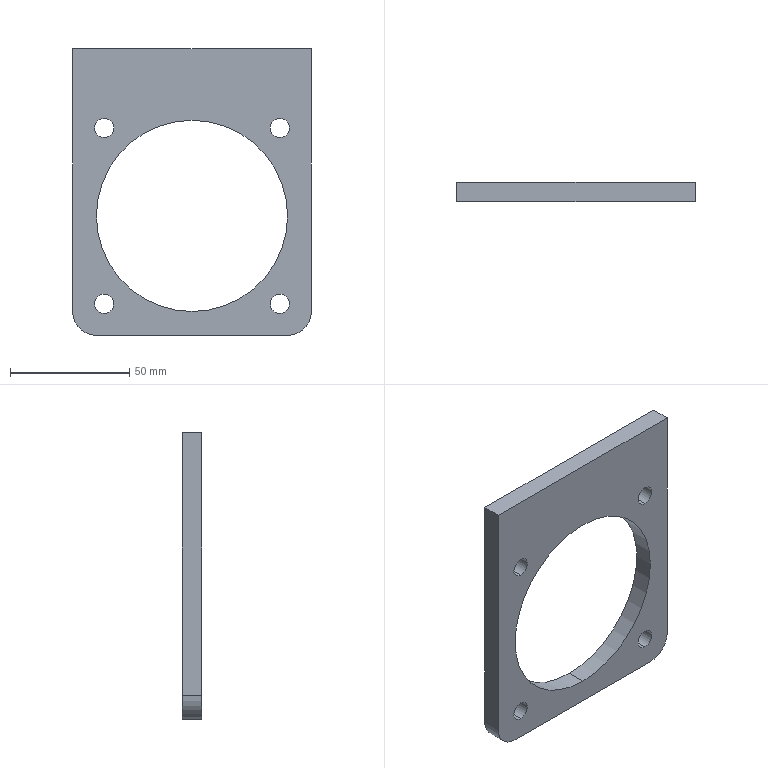Part | SolidWorks | features CirPattern 1, Extrusion 1, Fillet 1, HoleWzd 1, ICE 1 | 1 solid | 18 faces | box 100 x 8 x 120 mm | volume 53836 mm3 | cylinder 12 | plane 6 | commonest cylinder face diameters 8 x8 20 x2 80 x2
STEP:
#1=CARTESIAN_POINT('',(36.77,0.,-50.77));
#2=VERTEX_POINT('',#1);
#3=CARTESIAN_POINT('',(36.77,0.,-42.77));
#4=VERTEX_POINT('',#3);
#5=CARTESIAN_POINT('',(36.77,0.,-46.77));
#6=DIRECTION('',(0.,1.,0.));
#7=DIRECTION('',(0.,0.,1.));
#8=AXIS2_PLACEMENT_3D('',#5,#6,#7);
#9=CIRCLE('',#8,4.);
#10=EDGE_CURVE('',#2,#4,#9,.T.);
#11=ORIENTED_EDGE('',*,*,#10,.F.);
#12=CARTESIAN_POINT('',(36.77,8.,-50.77));
#13=VERTEX_POINT('',#12);
#14=CARTESIAN_POINT('',(36.77,8.,-50.77));
#15=DIRECTION('',(0.,1.,0.));
#16=VECTOR('',#15,1000.);
#17=LINE('',#14,#16);
#18=EDGE_CURVE('',#2,#13,#17,.T.);
#19=ORIENTED_EDGE('',*,*,#18,.T.);
#20=CARTESIAN_POINT('',(36.77,8.,-42.77));
#21=VERTEX_POINT('',#20);
#22=CARTESIAN_POINT('',(36.77,8.,-46.77));
#23=DIRECTION('',(0.,1.,0.));
#24=DIRECTION('',(0.,0.,1.));
#25=AXIS2_PLACEMENT_3D('',#22,#23,#24);
#26=CIRCLE('',#25,4.);
#27=EDGE_CURVE('',#13,#21,#26,.T.);
#28=ORIENTED_EDGE('',*,*,#27,.T.);
#29=CARTESIAN_POINT('',(36.77,8.,-42.77));
#30=DIRECTION('',(0.,1.,0.));
#31=VECTOR('',#30,1000.);
#32=LINE('',#29,#31);
#33=EDGE_CURVE('',#4,#21,#32,.T.);
#34=ORIENTED_EDGE('',*,*,#33,.F.);
#35=EDGE_LOOP('',(#11,#19,#28,#34));
#36=FACE_OUTER_BOUND('',#35,.T.);
#37=CARTESIAN_POINT('',(36.77,8.,-46.77));
#38=DIRECTION('',(0.,1.,0.));
#39=DIRECTION('',(0.,0.,1.));
#40=AXIS2_PLACEMENT_3D('',#37,#38,#39);
#41=CYLINDRICAL_SURFACE('',#40,4.);
#42=ADVANCED_FACE('',(#36),#41,.F.);
#43=CARTESIAN_POINT('',(36.77,0.,22.77));
#44=VERTEX_POINT('',#43);
#45=CARTESIAN_POINT('',(36.77,0.,30.77));
#46=VERTEX_POINT('',#45);
#47=CARTESIAN_POINT('',(36.77,0.,26.77));
#48=DIRECTION('',(0.,1.,0.));
#49=DIRECTION('',(0.,0.,1.));
#50=AXIS2_PLACEMENT_3D('',#47,#48,#49);
#51=CIRCLE('',#50,4.);
#52=EDGE_CURVE('',#44,#46,#51,.T.);
#53=ORIENTED_EDGE('',*,*,#52,.F.);
#54=CARTESIAN_POINT('',(36.77,8.,22.77));
#55=VERTEX_POINT('',#54);
#56=CARTESIAN_POINT('',(36.77,8.,22.77));
#57=DIRECTION('',(0.,1.,0.));
#58=VECTOR('',#57,1000.);
#59=LINE('',#56,#58);
#60=EDGE_CURVE('',#44,#55,#59,.T.);
#61=ORIENTED_EDGE('',*,*,#60,.T.);
#62=CARTESIAN_POINT('',(36.77,8.,30.77));
#63=VERTEX_POINT('',#62);
#64=CARTESIAN_POINT('',(36.77,8.,26.77));
#65=DIRECTION('',(0.,1.,0.));
#66=DIRECTION('',(0.,0.,1.));
#67=AXIS2_PLACEMENT_3D('',#64,#65,#66);
#68=CIRCLE('',#67,4.);
#69=EDGE_CURVE('',#55,#63,#68,.T.);
#70=ORIENTED_EDGE('',*,*,#69,.T.);
#71=CARTESIAN_POINT('',(36.77,8.,30.77));
#72=DIRECTION('',(0.,1.,0.));
#73=VECTOR('',#72,1000.);
#74=LINE('',#71,#73);
#75=EDGE_CURVE('',#46,#63,#74,.T.);
#76=ORIENTED_EDGE('',*,*,#75,.F.);
#77=EDGE_LOOP('',(#53,#61,#70,#76));
#78=FACE_OUTER_BOUND('',#77,.T.);
#79=CARTESIAN_POINT('',(36.77,8.,26.77));
#80=DIRECTION('',(0.,1.,0.));
#81=DIRECTION('',(0.,0.,1.));
#82=AXIS2_PLACEMENT_3D('',#79,#80,#81);
#83=CYLINDRICAL_SURFACE('',#82,4.);
#84=ADVANCED_FACE('',(#78),#83,.F.);
#85=CARTESIAN_POINT('',(-36.77,0.,22.77));
#86=VERTEX_POINT('',#85);
#87=CARTESIAN_POINT('',(-36.77,0.,30.77));
#88=VERTEX_POINT('',#87);
#89=CARTESIAN_POINT('',(-36.77,0.,26.77));
#90=DIRECTION('',(0.,1.,0.));
#91=DIRECTION('',(0.,0.,1.));
#92=AXIS2_PLACEMENT_3D('',#89,#90,#91);
#93=CIRCLE('',#92,4.);
#94=EDGE_CURVE('',#86,#88,#93,.T.);
#95=ORIENTED_EDGE('',*,*,#94,.F.);
#96=CARTESIAN_POINT('',(-36.77,8.,22.77));
#97=VERTEX_POINT('',#96);
#98=CARTESIAN_POINT('',(-36.77,8.,22.77));
#99=DIRECTION('',(0.,1.,0.));
#100=VECTOR('',#99,1000.);
#101=LINE('',#98,#100);
#102=EDGE_CURVE('',#86,#97,#101,.T.);
#103=ORIENTED_EDGE('',*,*,#102,.T.);
#104=CARTESIAN_POINT('',(-36.77,8.,30.77));
#105=VERTEX_POINT('',#104);
#106=CARTESIAN_POINT('',(-36.77,8.,26.77));
#107=DIRECTION('',(0.,1.,0.));
#108=DIRECTION('',(0.,0.,1.));
#109=AXIS2_PLACEMENT_3D('',#106,#107,#108);
#110=CIRCLE('',#109,4.);
#111=EDGE_CURVE('',#97,#105,#110,.T.);
#112=ORIENTED_EDGE('',*,*,#111,.T.);
#113=CARTESIAN_POINT('',(-36.77,8.,30.77));
#114=DIRECTION('',(0.,1.,0.));
#115=VECTOR('',#114,1000.);
#116=LINE('',#113,#115);
#117=EDGE_CURVE('',#88,#105,#116,.T.);
#118=ORIENTED_EDGE('',*,*,#117,.F.);
#119=EDGE_LOOP('',(#95,#103,#112,#118));
#120=FACE_OUTER_BOUND('',#119,.T.);
#121=CARTESIAN_POINT('',(-36.77,8.,26.77));
#122=DIRECTION('',(0.,1.,0.));
#123=DIRECTION('',(0.,0.,1.));
#124=AXIS2_PLACEMENT_3D('',#121,#122,#123);
#125=CYLINDRICAL_SURFACE('',#124,4.);
#126=ADVANCED_FACE('',(#120),#125,.F.);
#127=CARTESIAN_POINT('',(-36.77,0.,-50.77));
#128=VERTEX_POINT('',#127);
#129=CARTESIAN_POINT('',(-36.77,0.,-42.77));
#130=VERTEX_POINT('',#129);
#131=CARTESIAN_POINT('',(-36.77,0.,-46.77));
#132=DIRECTION('',(0.,1.,0.));
#133=DIRECTION('',(0.,0.,1.));
#134=AXIS2_PLACEMENT_3D('',#131,#132,#133);
#135=CIRCLE('',#134,4.);
#136=EDGE_CURVE('',#128,#130,#135,.T.);
#137=ORIENTED_EDGE('',*,*,#136,.F.);
#138=CARTESIAN_POINT('',(-36.77,8.,-50.77));
#139=VERTEX_POINT('',#138);
#140=CARTESIAN_POINT('',(-36.77,8.,-50.77));
#141=DIRECTION('',(0.,1.,0.));
#142=VECTOR('',#141,1000.);
#143=LINE('',#140,#142);
#144=EDGE_CURVE('',#128,#139,#143,.T.);
#145=ORIENTED_EDGE('',*,*,#144,.T.);
#146=CARTESIAN_POINT('',(-36.77,8.,-42.77));
#147=VERTEX_POINT('',#146);
#148=CARTESIAN_POINT('',(-36.77,8.,-46.77));
#149=DIRECTION('',(0.,1.,0.));
#150=DIRECTION('',(0.,0.,1.));
#151=AXIS2_PLACEMENT_3D('',#148,#149,#150);
#152=CIRCLE('',#151,4.);
#153=EDGE_CURVE('',#139,#147,#152,.T.);
#154=ORIENTED_EDGE('',*,*,#153,.T.);
#155=CARTESIAN_POINT('',(-36.77,8.,-42.77));
#156=DIRECTION('',(0.,1.,0.));
#157=VECTOR('',#156,1000.);
#158=LINE('',#155,#157);
#159=EDGE_CURVE('',#130,#147,#158,.T.);
#160=ORIENTED_EDGE('',*,*,#159,.F.);
#161=EDGE_LOOP('',(#137,#145,#154,#160));
#162=FACE_OUTER_BOUND('',#161,.T.);
#163=CARTESIAN_POINT('',(-36.77,8.,-46.77));
#164=DIRECTION('',(0.,1.,0.));
#165=DIRECTION('',(0.,0.,1.));
#166=AXIS2_PLACEMENT_3D('',#163,#164,#165);
#167=CYLINDRICAL_SURFACE('',#166,4.);
#168=ADVANCED_FACE('',(#162),#167,.F.);
#169=CARTESIAN_POINT('',(0.,0.,30.));
#170=VERTEX_POINT('',#169);
#171=CARTESIAN_POINT('',(0.,0.,-50.));
#172=VERTEX_POINT('',#171);
#173=CARTESIAN_POINT('',(0.,0.,-10.));
#174=DIRECTION('',(0.,-1.,0.));
#175=DIRECTION('',(0.,0.,1.));
#176=AXIS2_PLACEMENT_3D('',#173,#174,#175);
#177=CIRCLE('',#176,40.);
#178=EDGE_CURVE('',#170,#172,#177,.T.);
#179=ORIENTED_EDGE('',*,*,#178,.T.);
#180=CARTESIAN_POINT('',(0.,8.,-50.));
#181=VERTEX_POINT('',#180);
#182=CARTESIAN_POINT('',(0.,-0.001,-50.));
#183=DIRECTION('',(0.,1.,0.));
#184=VECTOR('',#183,1000.);
#185=LINE('',#182,#184);
#186=EDGE_CURVE('',#172,#181,#185,.T.);
#187=ORIENTED_EDGE('',*,*,#186,.T.);
#188=CARTESIAN_POINT('',(0.,8.,30.));
#189=VERTEX_POINT('',#188);
#190=CARTESIAN_POINT('',(0.,8.,-10.));
#191=DIRECTION('',(0.,1.,0.));
#192=DIRECTION('',(0.,0.,1.));
#193=AXIS2_PLACEMENT_3D('',#190,#191,#192);
#194=CIRCLE('',#193,40.);
#195=EDGE_CURVE('',#181,#189,#194,.T.);
#196=ORIENTED_EDGE('',*,*,#195,.T.);
#197=CARTESIAN_POINT('',(0.,-0.001,30.));
#198=DIRECTION('',(0.,1.,0.));
#199=VECTOR('',#198,1000.);
#200=LINE('',#197,#199);
#201=EDGE_CURVE('',#170,#189,#200,.T.);
#202=ORIENTED_EDGE('',*,*,#201,.F.);
#203=EDGE_LOOP('',(#179,#187,#196,#202));
#204=FACE_OUTER_BOUND('',#203,.T.);
#205=CARTESIAN_POINT('',(0.,-0.001,-10.));
#206=DIRECTION('',(0.,1.,0.));
#207=DIRECTION('',(0.,0.,1.));
#208=AXIS2_PLACEMENT_3D('',#205,#206,#207);
#209=CYLINDRICAL_SURFACE('',#208,40.);
#210=ADVANCED_FACE('',(#204),#209,.F.);
#211=CARTESIAN_POINT('',(-50.,8.,-50.));
#212=VERTEX_POINT('',#211);
#213=CARTESIAN_POINT('',(-50.,8.,60.));
#214=VERTEX_POINT('',#213);
#215=CARTESIAN_POINT('',(-50.,8.,60.));
#216=DIRECTION('',(0.,0.,1.));
#217=VECTOR('',#216,1000.);
#218=LINE('',#215,#217);
#219=EDGE_CURVE('',#212,#214,#218,.T.);
#220=ORIENTED_EDGE('',*,*,#219,.F.);
#221=CARTESIAN_POINT('',(-50.,0.,-50.));
#222=VERTEX_POINT('',#221);
#223=CARTESIAN_POINT('',(-50.,8.,-50.));
#224=DIRECTION('',(0.,-1.,0.));
#225=VECTOR('',#224,1000.);
#226=LINE('',#223,#225);
#227=EDGE_CURVE('',#212,#222,#226,.T.);
#228=ORIENTED_EDGE('',*,*,#227,.T.);
#229=CARTESIAN_POINT('',(-50.,0.,60.));
#230=VERTEX_POINT('',#229);
#231=CARTESIAN_POINT('',(-50.,0.,60.));
#232=DIRECTION('',(0.,0.,1.));
#233=VECTOR('',#232,1000.);
#234=LINE('',#231,#233);
#235=EDGE_CURVE('',#222,#230,#234,.T.);
#236=ORIENTED_EDGE('',*,*,#235,.T.);
#237=CARTESIAN_POINT('',(-50.,8.,60.));
#238=DIRECTION('',(0.,-1.,0.));
#239=VECTOR('',#238,1000.);
#240=LINE('',#237,#239);
#241=EDGE_CURVE('',#214,#230,#240,.T.);
#242=ORIENTED_EDGE('',*,*,#241,.F.);
#243=EDGE_LOOP('',(#220,#228,#236,#242));
#244=FACE_OUTER_BOUND('',#243,.T.);
#245=CARTESIAN_POINT('',(-50.,8.,60.));
#246=DIRECTION('',(1.,0.,0.));
#247=DIRECTION('',(0.,0.,-1.));
#248=AXIS2_PLACEMENT_3D('',#245,#246,#247);
#249=PLANE('',#248);
#250=ADVANCED_FACE('',(#244),#249,.F.);
#251=CARTESIAN_POINT('',(50.,0.,60.));
#252=VERTEX_POINT('',#251);
#253=CARTESIAN_POINT('',(50.,0.,60.));
#254=DIRECTION('',(1.,0.,0.));
#255=VECTOR('',#254,1000.);
#256=LINE('',#253,#255);
#257=EDGE_CURVE('',#230,#252,#256,.T.);
#258=ORIENTED_EDGE('',*,*,#257,.T.);
#259=CARTESIAN_POINT('',(50.,8.,60.));
#260=VERTEX_POINT('',#259);
#261=CARTESIAN_POINT('',(50.,8.,60.));
#262=DIRECTION('',(0.,-1.,0.));
#263=VECTOR('',#262,1000.);
#264=LINE('',#261,#263);
#265=EDGE_CURVE('',#260,#252,#264,.T.);
#266=ORIENTED_EDGE('',*,*,#265,.F.);
#267=CARTESIAN_POINT('',(50.,8.,60.));
#268=DIRECTION('',(1.,0.,0.));
#269=VECTOR('',#268,1000.);
#270=LINE('',#267,#269);
#271=EDGE_CURVE('',#214,#260,#270,.T.);
#272=ORIENTED_EDGE('',*,*,#271,.F.);
#273=ORIENTED_EDGE('',*,*,#241,.T.);
#274=EDGE_LOOP('',(#258,#266,#272,#273));
#275=FACE_OUTER_BOUND('',#274,.T.);
#276=CARTESIAN_POINT('',(50.,8.,60.));
#277=DIRECTION('',(0.,0.,-1.));
#278=DIRECTION('',(-1.,0.,0.));
#279=AXIS2_PLACEMENT_3D('',#276,#277,#278);
#280=PLANE('',#279);
#281=ADVANCED_FACE('',(#275),#280,.F.);
#282=CARTESIAN_POINT('',(50.,0.,-50.));
#283=VERTEX_POINT('',#282);
#284=CARTESIAN_POINT('',(50.,0.,60.));
#285=DIRECTION('',(0.,0.,-1.));
#286=VECTOR('',#285,1000.);
#287=LINE('',#284,#286);
#288=EDGE_CURVE('',#252,#283,#287,.T.);
#289=ORIENTED_EDGE('',*,*,#288,.T.);
#290=CARTESIAN_POINT('',(50.,8.,-50.));
#291=VERTEX_POINT('',#290);
#292=CARTESIAN_POINT('',(50.,8.,-50.));
#293=DIRECTION('',(0.,1.,0.));
#294=VECTOR('',#293,1000.);
#295=LINE('',#292,#294);
#296=EDGE_CURVE('',#283,#291,#295,.T.);
#297=ORIENTED_EDGE('',*,*,#296,.T.);
#298=CARTESIAN_POINT('',(50.,8.,60.));
#299=DIRECTION('',(0.,0.,-1.));
#300=VECTOR('',#299,1000.);
#301=LINE('',#298,#300);
#302=EDGE_CURVE('',#260,#291,#301,.T.);
#303=ORIENTED_EDGE('',*,*,#302,.F.);
#304=ORIENTED_EDGE('',*,*,#265,.T.);
#305=EDGE_LOOP('',(#289,#297,#303,#304));
#306=FACE_OUTER_BOUND('',#305,.T.);
#307=CARTESIAN_POINT('',(50.,8.,60.));
#308=DIRECTION('',(-1.,0.,0.));
#309=DIRECTION('',(0.,0.,1.));
#310=AXIS2_PLACEMENT_3D('',#307,#308,#309);
#311=PLANE('',#310);
#312=ADVANCED_FACE('',(#306),#311,.F.);
#313=CARTESIAN_POINT('',(40.,8.,-60.));
#314=VERTEX_POINT('',#313);
#315=CARTESIAN_POINT('',(-40.,8.,-60.));
#316=VERTEX_POINT('',#315);
#317=CARTESIAN_POINT('',(50.,8.,-60.));
#318=DIRECTION('',(-1.,0.,0.));
#319=VECTOR('',#318,1000.);
#320=LINE('',#317,#319);
#321=EDGE_CURVE('',#314,#316,#320,.T.);
#322=ORIENTED_EDGE('',*,*,#321,.F.);
#323=CARTESIAN_POINT('',(40.,0.,-60.));
#324=VERTEX_POINT('',#323);
#325=CARTESIAN_POINT('',(40.,8.,-60.));
#326=DIRECTION('',(0.,-1.,0.));
#327=VECTOR('',#326,1000.);
#328=LINE('',#325,#327);
#329=EDGE_CURVE('',#314,#324,#328,.T.);
#330=ORIENTED_EDGE('',*,*,#329,.T.);
#331=CARTESIAN_POINT('',(-40.,0.,-60.));
#332=VERTEX_POINT('',#331);
#333=CARTESIAN_POINT('',(50.,0.,-60.));
#334=DIRECTION('',(-1.,0.,0.));
#335=VECTOR('',#334,1000.);
#336=LINE('',#333,#335);
#337=EDGE_CURVE('',#324,#332,#336,.T.);
#338=ORIENTED_EDGE('',*,*,#337,.T.);
#339=CARTESIAN_POINT('',(-40.,8.,-60.));
#340=DIRECTION('',(0.,1.,0.));
#341=VECTOR('',#340,1000.);
#342=LINE('',#339,#341);
#343=EDGE_CURVE('',#332,#316,#342,.T.);
#344=ORIENTED_EDGE('',*,*,#343,.T.);
#345=EDGE_LOOP('',(#322,#330,#338,#344));
#346=FACE_OUTER_BOUND('',#345,.T.);
#347=CARTESIAN_POINT('',(50.,8.,-60.));
#348=DIRECTION('',(0.,0.,1.));
#349=DIRECTION('',(1.,0.,0.));
#350=AXIS2_PLACEMENT_3D('',#347,#348,#349);
#351=PLANE('',#350);
#352=ADVANCED_FACE('',(#346),#351,.F.);
#353=CARTESIAN_POINT('',(36.77,8.,-46.77));
#354=DIRECTION('',(0.,1.,0.));
#355=DIRECTION('',(0.,0.,1.));
#356=AXIS2_PLACEMENT_3D('',#353,#354,#355);
#357=CIRCLE('',#356,4.);
#358=EDGE_CURVE('',#21,#13,#357,.T.);
#359=ORIENTED_EDGE('',*,*,#358,.F.);
#360=ORIENTED_EDGE('',*,*,#27,.F.);
#361=EDGE_LOOP('',(#359,#360));
#362=FACE_BOUND('',#361,.T.);
#363=CARTESIAN_POINT('',(36.77,8.,26.77));
#364=DIRECTION('',(0.,1.,0.));
#365=DIRECTION('',(0.,0.,1.));
#366=AXIS2_PLACEMENT_3D('',#363,#364,#365);
#367=CIRCLE('',#366,4.);
#368=EDGE_CURVE('',#63,#55,#367,.T.);
#369=ORIENTED_EDGE('',*,*,#368,.F.);
#370=ORIENTED_EDGE('',*,*,#69,.F.);
#371=EDGE_LOOP('',(#369,#370));
#372=FACE_BOUND('',#371,.T.);
#373=CARTESIAN_POINT('',(-36.77,8.,26.77));
#374=DIRECTION('',(0.,1.,0.));
#375=DIRECTION('',(0.,0.,1.));
#376=AXIS2_PLACEMENT_3D('',#373,#374,#375);
#377=CIRCLE('',#376,4.);
#378=EDGE_CURVE('',#105,#97,#377,.T.);
#379=ORIENTED_EDGE('',*,*,#378,.F.);
#380=ORIENTED_EDGE('',*,*,#111,.F.);
#381=EDGE_LOOP('',(#379,#380));
#382=FACE_BOUND('',#381,.T.);
#383=CARTESIAN_POINT('',(-36.77,8.,-46.77));
#384=DIRECTION('',(0.,1.,0.));
#385=DIRECTION('',(0.,0.,1.));
#386=AXIS2_PLACEMENT_3D('',#383,#384,#385);
#387=CIRCLE('',#386,4.);
#388=EDGE_CURVE('',#147,#139,#387,.T.);
#389=ORIENTED_EDGE('',*,*,#388,.F.);
#390=ORIENTED_EDGE('',*,*,#153,.F.);
#391=EDGE_LOOP('',(#389,#390));
#392=FACE_BOUND('',#391,.T.);
#393=CARTESIAN_POINT('',(0.,8.,-10.));
#394=DIRECTION('',(0.,1.,0.));
#395=DIRECTION('',(0.,0.,1.));
#396=AXIS2_PLACEMENT_3D('',#393,#394,#395);
#397=CIRCLE('',#396,40.);
#398=EDGE_CURVE('',#189,#181,#397,.T.);
#399=ORIENTED_EDGE('',*,*,#398,.F.);
#400=ORIENTED_EDGE('',*,*,#195,.F.);
#401=EDGE_LOOP('',(#399,#400));
#402=FACE_BOUND('',#401,.T.);
#403=ORIENTED_EDGE('',*,*,#302,.T.);
#404=CARTESIAN_POINT('',(40.,8.,-50.));
#405=DIRECTION('',(0.,1.,0.));
#406=DIRECTION('',(0.,0.,1.));
#407=AXIS2_PLACEMENT_3D('',#404,#405,#406);
#408=CIRCLE('',#407,10.);
#409=EDGE_CURVE('',#291,#314,#408,.T.);
#410=ORIENTED_EDGE('',*,*,#409,.T.);
#411=ORIENTED_EDGE('',*,*,#321,.T.);
#412=CARTESIAN_POINT('',(-40.,8.,-50.));
#413=DIRECTION('',(0.,1.,0.));
#414=DIRECTION('',(0.,0.,1.));
#415=AXIS2_PLACEMENT_3D('',#412,#413,#414);
#416=CIRCLE('',#415,10.);
#417=EDGE_CURVE('',#316,#212,#416,.T.);
#418=ORIENTED_EDGE('',*,*,#417,.T.);
#419=ORIENTED_EDGE('',*,*,#219,.T.);
#420=ORIENTED_EDGE('',*,*,#271,.T.);
#421=EDGE_LOOP('',(#403,#410,#411,#418,#419,#420));
#422=FACE_OUTER_BOUND('',#421,.T.);
#423=CARTESIAN_POINT('',(0.,8.,0.));
#424=DIRECTION('',(0.,1.,0.));
#425=DIRECTION('',(0.,0.,1.));
#426=AXIS2_PLACEMENT_3D('',#423,#424,#425);
#427=PLANE('',#426);
#428=ADVANCED_FACE('',(#362,#372,#382,#392,#402,#422),#427,.T.);
#429=CARTESIAN_POINT('',(36.77,0.,-46.77));
#430=DIRECTION('',(0.,1.,0.));
#431=DIRECTION('',(0.,0.,1.));
#432=AXIS2_PLACEMENT_3D('',#429,#430,#431);
#433=CIRCLE('',#432,4.);
#434=EDGE_CURVE('',#4,#2,#433,.T.);
#435=ORIENTED_EDGE('',*,*,#434,.T.);
#436=ORIENTED_EDGE('',*,*,#10,.T.);
#437=EDGE_LOOP('',(#435,#436));
#438=FACE_BOUND('',#437,.T.);
#439=CARTESIAN_POINT('',(36.77,0.,26.77));
#440=DIRECTION('',(0.,1.,0.));
#441=DIRECTION('',(0.,0.,1.));
#442=AXIS2_PLACEMENT_3D('',#439,#440,#441);
#443=CIRCLE('',#442,4.);
#444=EDGE_CURVE('',#46,#44,#443,.T.);
#445=ORIENTED_EDGE('',*,*,#444,.T.);
#446=ORIENTED_EDGE('',*,*,#52,.T.);
#447=EDGE_LOOP('',(#445,#446));
#448=FACE_BOUND('',#447,.T.);
#449=CARTESIAN_POINT('',(-36.77,0.,26.77));
#450=DIRECTION('',(0.,1.,0.));
#451=DIRECTION('',(0.,0.,1.));
#452=AXIS2_PLACEMENT_3D('',#449,#450,#451);
#453=CIRCLE('',#452,4.);
#454=EDGE_CURVE('',#88,#86,#453,.T.);
#455=ORIENTED_EDGE('',*,*,#454,.T.);
#456=ORIENTED_EDGE('',*,*,#94,.T.);
#457=EDGE_LOOP('',(#455,#456));
#458=FACE_BOUND('',#457,.T.);
#459=CARTESIAN_POINT('',(-36.77,0.,-46.77));
#460=DIRECTION('',(0.,1.,0.));
#461=DIRECTION('',(0.,0.,1.));
#462=AXIS2_PLACEMENT_3D('',#459,#460,#461);
#463=CIRCLE('',#462,4.);
#464=EDGE_CURVE('',#130,#128,#463,.T.);
#465=ORIENTED_EDGE('',*,*,#464,.T.);
#466=ORIENTED_EDGE('',*,*,#136,.T.);
#467=EDGE_LOOP('',(#465,#466));
#468=FACE_BOUND('',#467,.T.);
#469=ORIENTED_EDGE('',*,*,#178,.F.);
#470=CARTESIAN_POINT('',(0.,0.,-10.));
#471=DIRECTION('',(0.,-1.,0.));
#472=DIRECTION('',(0.,0.,1.));
#473=AXIS2_PLACEMENT_3D('',#470,#471,#472);
#474=CIRCLE('',#473,40.);
#475=EDGE_CURVE('',#172,#170,#474,.T.);
#476=ORIENTED_EDGE('',*,*,#475,.F.);
#477=EDGE_LOOP('',(#469,#476));
#478=FACE_BOUND('',#477,.T.);
#479=ORIENTED_EDGE('',*,*,#337,.F.);
#480=CARTESIAN_POINT('',(40.,0.,-50.));
#481=DIRECTION('',(0.,-1.,0.));
#482=DIRECTION('',(0.,0.,1.));
#483=AXIS2_PLACEMENT_3D('',#480,#481,#482);
#484=CIRCLE('',#483,10.);
#485=EDGE_CURVE('',#324,#283,#484,.T.);
#486=ORIENTED_EDGE('',*,*,#485,.T.);
#487=ORIENTED_EDGE('',*,*,#288,.F.);
#488=ORIENTED_EDGE('',*,*,#257,.F.);
#489=ORIENTED_EDGE('',*,*,#235,.F.);
#490=CARTESIAN_POINT('',(-40.,0.,-50.));
#491=DIRECTION('',(0.,-1.,0.));
#492=DIRECTION('',(0.,0.,1.));
#493=AXIS2_PLACEMENT_3D('',#490,#491,#492);
#494=CIRCLE('',#493,10.);
#495=EDGE_CURVE('',#222,#332,#494,.T.);
#496=ORIENTED_EDGE('',*,*,#495,.T.);
#497=EDGE_LOOP('',(#479,#486,#487,#488,#489,#496));
#498=FACE_OUTER_BOUND('',#497,.T.);
#499=CARTESIAN_POINT('',(0.,0.,0.));
#500=DIRECTION('',(0.,1.,0.));
#501=DIRECTION('',(0.,0.,1.));
#502=AXIS2_PLACEMENT_3D('',#499,#500,#501);
#503=PLANE('',#502);
#504=ADVANCED_FACE('',(#438,#448,#458,#468,#478,#498),#503,.F.);
#505=ORIENTED_EDGE('',*,*,#409,.F.);
#506=ORIENTED_EDGE('',*,*,#296,.F.);
#507=ORIENTED_EDGE('',*,*,#485,.F.);
#508=ORIENTED_EDGE('',*,*,#329,.F.);
#509=EDGE_LOOP('',(#505,#506,#507,#508));
#510=FACE_OUTER_BOUND('',#509,.T.);
#511=CARTESIAN_POINT('',(40.,8.,-50.));
#512=DIRECTION('',(0.,-1.,0.));
#513=DIRECTION('',(0.,0.,-1.));
#514=AXIS2_PLACEMENT_3D('',#511,#512,#513);
#515=CYLINDRICAL_SURFACE('',#514,10.);
#516=ADVANCED_FACE('',(#510),#515,.T.);
#517=ORIENTED_EDGE('',*,*,#417,.F.);
#518=ORIENTED_EDGE('',*,*,#343,.F.);
#519=ORIENTED_EDGE('',*,*,#495,.F.);
#520=ORIENTED_EDGE('',*,*,#227,.F.);
#521=EDGE_LOOP('',(#517,#518,#519,#520));
#522=FACE_OUTER_BOUND('',#521,.T.);
#523=CARTESIAN_POINT('',(-40.,8.,-50.));
#524=DIRECTION('',(0.,-1.,0.));
#525=DIRECTION('',(0.,0.,-1.));
#526=AXIS2_PLACEMENT_3D('',#523,#524,#525);
#527=CYLINDRICAL_SURFACE('',#526,10.);
#528=ADVANCED_FACE('',(#522),#527,.T.);
#529=ORIENTED_EDGE('',*,*,#186,.F.);
#530=ORIENTED_EDGE('',*,*,#475,.T.);
#531=ORIENTED_EDGE('',*,*,#201,.T.);
#532=ORIENTED_EDGE('',*,*,#398,.T.);
#533=EDGE_LOOP('',(#529,#530,#531,#532));
#534=FACE_OUTER_BOUND('',#533,.T.);
#535=CARTESIAN_POINT('',(0.,-0.001,-10.));
#536=DIRECTION('',(0.,1.,0.));
#537=DIRECTION('',(0.,0.,1.));
#538=AXIS2_PLACEMENT_3D('',#535,#536,#537);
#539=CYLINDRICAL_SURFACE('',#538,40.);
#540=ADVANCED_FACE('',(#534),#539,.F.);
#541=ORIENTED_EDGE('',*,*,#144,.F.);
#542=ORIENTED_EDGE('',*,*,#464,.F.);
#543=ORIENTED_EDGE('',*,*,#159,.T.);
#544=ORIENTED_EDGE('',*,*,#388,.T.);
#545=EDGE_LOOP('',(#541,#542,#543,#544));
#546=FACE_OUTER_BOUND('',#545,.T.);
#547=CARTESIAN_POINT('',(-36.77,8.,-46.77));
#548=DIRECTION('',(0.,1.,0.));
#549=DIRECTION('',(0.,0.,1.));
#550=AXIS2_PLACEMENT_3D('',#547,#548,#549);
#551=CYLINDRICAL_SURFACE('',#550,4.);
#552=ADVANCED_FACE('',(#546),#551,.F.);
#553=ORIENTED_EDGE('',*,*,#102,.F.);
#554=ORIENTED_EDGE('',*,*,#454,.F.);
#555=ORIENTED_EDGE('',*,*,#117,.T.);
#556=ORIENTED_EDGE('',*,*,#378,.T.);
#557=EDGE_LOOP('',(#553,#554,#555,#556));
#558=FACE_OUTER_BOUND('',#557,.T.);
#559=CARTESIAN_POINT('',(-36.77,8.,26.77));
#560=DIRECTION('',(0.,1.,0.));
#561=DIRECTION('',(0.,0.,1.));
#562=AXIS2_PLACEMENT_3D('',#559,#560,#561);
#563=CYLINDRICAL_SURFACE('',#562,4.);
#564=ADVANCED_FACE('',(#558),#563,.F.);
#565=ORIENTED_EDGE('',*,*,#60,.F.);
#566=ORIENTED_EDGE('',*,*,#444,.F.);
#567=ORIENTED_EDGE('',*,*,#75,.T.);
#568=ORIENTED_EDGE('',*,*,#368,.T.);
#569=EDGE_LOOP('',(#565,#566,#567,#568));
#570=FACE_OUTER_BOUND('',#569,.T.);
#571=CARTESIAN_POINT('',(36.77,8.,26.77));
#572=DIRECTION('',(0.,1.,0.));
#573=DIRECTION('',(0.,0.,1.));
#574=AXIS2_PLACEMENT_3D('',#571,#572,#573);
#575=CYLINDRICAL_SURFACE('',#574,4.);
#576=ADVANCED_FACE('',(#570),#575,.F.);
#577=ORIENTED_EDGE('',*,*,#18,.F.);
#578=ORIENTED_EDGE('',*,*,#434,.F.);
#579=ORIENTED_EDGE('',*,*,#33,.T.);
#580=ORIENTED_EDGE('',*,*,#358,.T.);
#581=EDGE_LOOP('',(#577,#578,#579,#580));
#582=FACE_OUTER_BOUND('',#581,.T.);
#583=CARTESIAN_POINT('',(36.77,8.,-46.77));
#584=DIRECTION('',(0.,1.,0.));
#585=DIRECTION('',(0.,0.,1.));
#586=AXIS2_PLACEMENT_3D('',#583,#584,#585);
#587=CYLINDRICAL_SURFACE('',#586,4.);
#588=ADVANCED_FACE('',(#582),#587,.F.);
#589=CLOSED_SHELL('',(#42,#84,#126,#168,#210,#250,#281,#312,#352,#428,#504,#516,#528,#540,#552,#564,#576,#588));
#590=MANIFOLD_SOLID_BREP('',#589);
#591=CARTESIAN_POINT('',(0.,0.,0.));
#592=DIRECTION('',(0.,0.,1.));
#593=DIRECTION('',(1.,0.,0.));
#594=AXIS2_PLACEMENT_3D('',#591,#592,#593);
#595=(LENGTH_UNIT()NAMED_UNIT(*)SI_UNIT(.MILLI.,.METRE.));
#596=UNCERTAINTY_MEASURE_WITH_UNIT(LENGTH_MEASURE(0.00001),#595,'','');
#597=(NAMED_UNIT(*)PLANE_ANGLE_UNIT()SI_UNIT($,.RADIAN.));
#598=(NAMED_UNIT(*)SI_UNIT($,.STERADIAN.)SOLID_ANGLE_UNIT());
#599=(GEOMETRIC_REPRESENTATION_CONTEXT(3)GLOBAL_UNCERTAINTY_ASSIGNED_CONTEXT((#596))GLOBAL_UNIT_ASSIGNED_CONTEXT((#595,#597,#598))REPRESENTATION_CONTEXT('',''));
#600=ADVANCED_BREP_SHAPE_REPRESENTATION('',(#590,#594),#599);